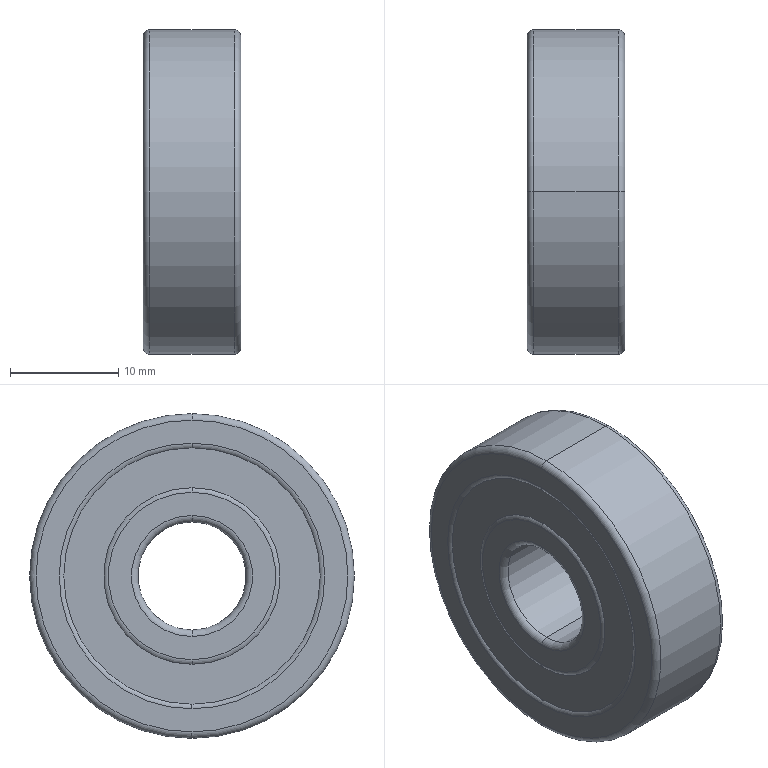Part | SolidWorks | features BaseBody 12 | 12 solids | 148 faces | box 9 x 30 x 30 mm | volume 4389 mm3 | cylinder 50 | sphere 44 | plane 28 | torus 26 | commonest cylinder face diameters 19 x19 21 x19 16.667 x4 23.333 x4 10 x2 30 x2